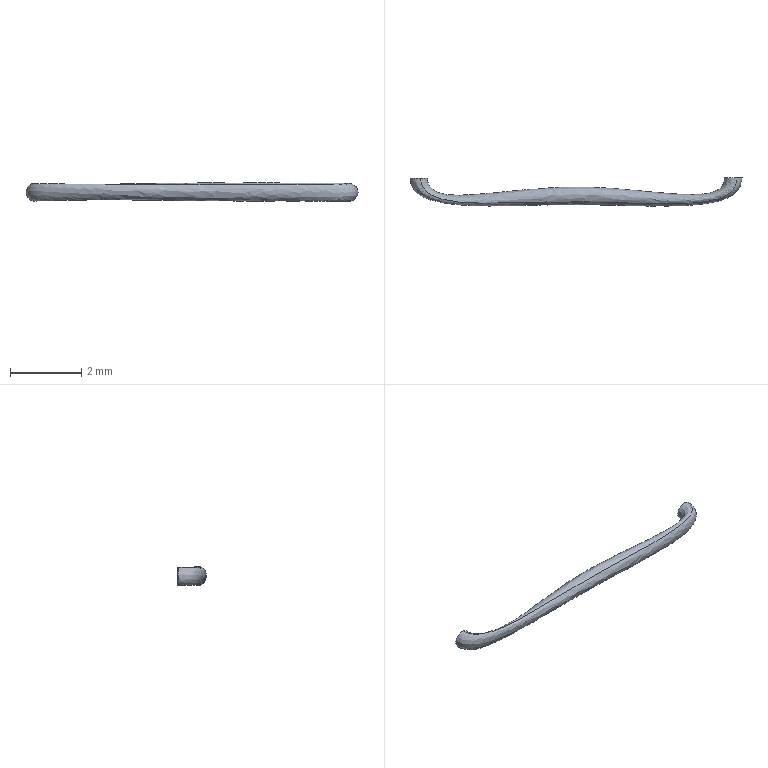Part | SolidWorks | features BaseBody 1 | 1 solid | 4 faces | box 9.341 x 0.7921 x 0.5174 mm | volume 1.419 mm3 | plane 2 | spline 2
STEP:
#1=CARTESIAN_POINT('',(346.48,392.468,97.127));
#2=VERTEX_POINT('',#1);
#3=CARTESIAN_POINT('',(346.268,392.468,96.674));
#4=VERTEX_POINT('',#3);
#5=CARTESIAN_POINT('',(346.48,392.468,97.127));
#6=CARTESIAN_POINT('',(346.486,392.468,97.124));
#7=CARTESIAN_POINT('',(346.498,392.468,97.117));
#8=CARTESIAN_POINT('',(346.515,392.468,97.107));
#9=CARTESIAN_POINT('',(346.531,392.468,97.095));
#10=CARTESIAN_POINT('',(346.581,392.468,97.051));
#11=CARTESIAN_POINT('',(346.622,392.469,96.975));
#12=CARTESIAN_POINT('',(346.626,392.469,96.871));
#13=CARTESIAN_POINT('',(346.602,392.469,96.785));
#14=CARTESIAN_POINT('',(346.545,392.468,96.709));
#15=CARTESIAN_POINT('',(346.461,392.468,96.66));
#16=CARTESIAN_POINT('',(346.365,392.468,96.644));
#17=CARTESIAN_POINT('',(346.298,392.468,96.66));
#18=CARTESIAN_POINT('',(346.268,392.468,96.674));
#19=B_SPLINE_CURVE_WITH_KNOTS('',3,(#5,#6,#7,#8,#9,#10,#11,#12,#13,#14,#15,#16,#17,#18),.UNSPECIFIED.,.F.,.F.,(4,1,1,1,1,1,1,1,1,1,1,4),(0.,0.025,0.05,0.075,0.1,0.3,0.4,0.5,0.625,0.75,0.875,1.),.UNSPECIFIED.);
#20=EDGE_CURVE('',#2,#4,#19,.T.);
#21=ORIENTED_EDGE('',*,*,#20,.T.);
#22=CARTESIAN_POINT('',(346.268,392.468,96.674));
#23=CARTESIAN_POINT('',(346.237,392.468,96.688));
#24=CARTESIAN_POINT('',(346.182,392.468,96.729));
#25=CARTESIAN_POINT('',(346.133,392.468,96.813));
#26=CARTESIAN_POINT('',(346.117,392.468,96.909));
#27=CARTESIAN_POINT('',(346.14,392.468,97.002));
#28=CARTESIAN_POINT('',(346.19,392.468,97.076));
#29=CARTESIAN_POINT('',(346.273,392.468,97.139));
#30=CARTESIAN_POINT('',(346.358,392.468,97.156));
#31=CARTESIAN_POINT('',(346.423,392.468,97.146));
#32=CARTESIAN_POINT('',(346.442,392.468,97.141));
#33=CARTESIAN_POINT('',(346.461,392.468,97.135));
#34=CARTESIAN_POINT('',(346.474,392.468,97.129));
#35=CARTESIAN_POINT('',(346.48,392.468,97.127));
#36=B_SPLINE_CURVE_WITH_KNOTS('',3,(#22,#23,#24,#25,#26,#27,#28,#29,#30,#31,#32,#33,#34,#35),.UNSPECIFIED.,.F.,.F.,(4,1,1,1,1,1,1,1,1,1,1,4),(0.,0.125,0.25,0.375,0.5,0.6,0.7,0.9,0.925,0.95,0.975,1.),.UNSPECIFIED.);
#37=EDGE_CURVE('',#4,#2,#36,.T.);
#38=ORIENTED_EDGE('',*,*,#37,.T.);
#39=EDGE_LOOP('',(#21,#38));
#40=FACE_OUTER_BOUND('',#39,.T.);
#41=CARTESIAN_POINT('',(346.374,392.468,96.9));
#42=DIRECTION('',(0.0009599,-1.,0.));
#43=DIRECTION('',(0.,0.,-1.));
#44=AXIS2_PLACEMENT_3D('',#41,#42,#43);
#45=PLANE('',#44);
#46=ADVANCED_FACE('',(#40),#45,.F.);
#47=CARTESIAN_POINT('',(337.585,392.46,97.145));
#48=VERTEX_POINT('',#47);
#49=CARTESIAN_POINT('',(337.481,392.46,96.656));
#50=VERTEX_POINT('',#49);
#51=CARTESIAN_POINT('',(337.585,392.46,97.145));
#52=CARTESIAN_POINT('',(337.591,392.46,97.143));
#53=CARTESIAN_POINT('',(337.605,392.46,97.14));
#54=CARTESIAN_POINT('',(337.624,392.46,97.133));
#55=CARTESIAN_POINT('',(337.642,392.46,97.125));
#56=CARTESIAN_POINT('',(337.7,392.46,97.094));
#57=CARTESIAN_POINT('',(337.757,392.46,97.029));
#58=CARTESIAN_POINT('',(337.785,392.46,96.929));
#59=CARTESIAN_POINT('',(337.781,392.46,96.84));
#60=CARTESIAN_POINT('',(337.743,392.46,96.753));
#61=CARTESIAN_POINT('',(337.672,392.46,96.686));
#62=CARTESIAN_POINT('',(337.582,392.46,96.648));
#63=CARTESIAN_POINT('',(337.514,392.46,96.649));
#64=CARTESIAN_POINT('',(337.481,392.46,96.656));
#65=B_SPLINE_CURVE_WITH_KNOTS('',3,(#51,#52,#53,#54,#55,#56,#57,#58,#59,#60,#61,#62,#63,#64),.UNSPECIFIED.,.F.,.F.,(4,1,1,1,1,1,1,1,1,1,1,4),(0.,0.025,0.05,0.075,0.1,0.3,0.4,0.5,0.625,0.75,0.875,1.),.UNSPECIFIED.);
#66=EDGE_CURVE('',#48,#50,#65,.T.);
#67=ORIENTED_EDGE('',*,*,#66,.T.);
#68=CARTESIAN_POINT('',(337.481,392.46,96.656));
#69=CARTESIAN_POINT('',(337.448,392.46,96.663));
#70=CARTESIAN_POINT('',(337.385,392.46,96.69));
#71=CARTESIAN_POINT('',(337.318,392.46,96.761));
#72=CARTESIAN_POINT('',(337.281,392.46,96.851));
#73=CARTESIAN_POINT('',(337.281,392.46,96.947));
#74=CARTESIAN_POINT('',(337.314,392.46,97.029));
#75=CARTESIAN_POINT('',(337.38,392.46,97.109));
#76=CARTESIAN_POINT('',(337.459,392.46,97.146));
#77=CARTESIAN_POINT('',(337.524,392.46,97.15));
#78=CARTESIAN_POINT('',(337.544,392.46,97.15));
#79=CARTESIAN_POINT('',(337.564,392.46,97.148));
#80=CARTESIAN_POINT('',(337.578,392.46,97.146));
#81=CARTESIAN_POINT('',(337.585,392.46,97.145));
#82=B_SPLINE_CURVE_WITH_KNOTS('',3,(#68,#69,#70,#71,#72,#73,#74,#75,#76,#77,#78,#79,#80,#81),.UNSPECIFIED.,.F.,.F.,(4,1,1,1,1,1,1,1,1,1,1,4),(0.,0.125,0.25,0.375,0.5,0.6,0.7,0.9,0.925,0.95,0.975,1.),.UNSPECIFIED.);
#83=EDGE_CURVE('',#50,#48,#82,.T.);
#84=ORIENTED_EDGE('',*,*,#83,.T.);
#85=EDGE_LOOP('',(#67,#84));
#86=FACE_OUTER_BOUND('',#85,.T.);
#87=CARTESIAN_POINT('',(337.533,392.46,96.9));
#88=DIRECTION('',(0.0009599,-1.,0.));
#89=DIRECTION('',(0.,0.,-1.));
#90=AXIS2_PLACEMENT_3D('',#87,#88,#89);
#91=PLANE('',#90);
#92=ADVANCED_FACE('',(#86),#91,.F.);
#93=CARTESIAN_POINT('',(337.481,392.46,96.656));
#94=CARTESIAN_POINT('',(337.482,391.517,96.656));
#95=CARTESIAN_POINT('',(342.031,392.705,96.768));
#96=CARTESIAN_POINT('',(346.269,391.557,96.674));
#97=CARTESIAN_POINT('',(346.268,392.468,96.674));
#98=B_SPLINE_CURVE_WITH_KNOTS('',3,(#93,#94,#95,#96,#97),.UNSPECIFIED.,.F.,.F.,(4,1,4),(0.,0.5,1.),.UNSPECIFIED.);
#99=EDGE_CURVE('',#50,#4,#98,.T.);
#100=ORIENTED_EDGE('',*,*,#99,.T.);
#101=ORIENTED_EDGE('',*,*,#20,.F.);
#102=CARTESIAN_POINT('',(346.48,392.468,97.127));
#103=CARTESIAN_POINT('',(346.481,391.466,97.127));
#104=CARTESIAN_POINT('',(341.874,392.138,97.077));
#105=CARTESIAN_POINT('',(337.586,391.489,97.145));
#106=CARTESIAN_POINT('',(337.585,392.46,97.145));
#107=B_SPLINE_CURVE_WITH_KNOTS('',3,(#102,#103,#104,#105,#106),.UNSPECIFIED.,.F.,.F.,(4,1,4),(0.,0.5,1.),.UNSPECIFIED.);
#108=EDGE_CURVE('',#2,#48,#107,.T.);
#109=ORIENTED_EDGE('',*,*,#108,.T.);
#110=ORIENTED_EDGE('',*,*,#83,.F.);
#111=EDGE_LOOP('',(#100,#101,#109,#110));
#112=FACE_OUTER_BOUND('',#111,.T.);
#113=CARTESIAN_POINT('',(337.606,392.553,97.141));
#114=CARTESIAN_POINT('',(337.469,391.473,97.142));
#115=CARTESIAN_POINT('',(341.873,392.18,97.093));
#116=CARTESIAN_POINT('',(346.619,391.448,97.134));
#117=CARTESIAN_POINT('',(346.458,392.572,97.133));
#118=CARTESIAN_POINT('',(337.601,392.553,97.142));
#119=CARTESIAN_POINT('',(337.464,391.471,97.144));
#120=CARTESIAN_POINT('',(341.873,392.173,97.087));
#121=CARTESIAN_POINT('',(346.624,391.446,97.132));
#122=CARTESIAN_POINT('',(346.463,392.572,97.131));
#123=CARTESIAN_POINT('',(337.589,392.554,97.145));
#124=CARTESIAN_POINT('',(337.451,391.468,97.147));
#125=CARTESIAN_POINT('',(341.873,392.157,97.073));
#126=CARTESIAN_POINT('',(346.635,391.443,97.128));
#127=CARTESIAN_POINT('',(346.474,392.572,97.126));
#128=CARTESIAN_POINT('',(337.57,392.554,97.148));
#129=CARTESIAN_POINT('',(337.432,391.462,97.151));
#130=CARTESIAN_POINT('',(341.874,392.133,97.05));
#131=CARTESIAN_POINT('',(346.652,391.438,97.119));
#132=CARTESIAN_POINT('',(346.491,392.573,97.117));
#133=CARTESIAN_POINT('',(337.55,392.555,97.15));
#134=CARTESIAN_POINT('',(337.411,391.456,97.154));
#135=CARTESIAN_POINT('',(341.876,392.111,97.025));
#136=CARTESIAN_POINT('',(346.67,391.433,97.109));
#137=CARTESIAN_POINT('',(346.508,392.574,97.106));
#138=CARTESIAN_POINT('',(337.53,392.555,97.15));
#139=CARTESIAN_POINT('',(337.391,391.451,97.155));
#140=CARTESIAN_POINT('',(341.878,392.09,97.));
#141=CARTESIAN_POINT('',(346.686,391.428,97.098));
#142=CARTESIAN_POINT('',(346.524,392.574,97.094));
#143=CARTESIAN_POINT('',(337.465,392.557,97.145));
#144=CARTESIAN_POINT('',(337.323,391.433,97.153));
#145=CARTESIAN_POINT('',(341.887,392.031,96.914));
#146=CARTESIAN_POINT('',(346.737,391.414,97.056));
#147=CARTESIAN_POINT('',(346.573,392.576,97.051));
#148=CARTESIAN_POINT('',(337.386,392.559,97.109));
#149=CARTESIAN_POINT('',(337.241,391.413,97.119));
#150=CARTESIAN_POINT('',(341.907,392.003,96.801));
#151=CARTESIAN_POINT('',(346.779,391.403,96.981));
#152=CARTESIAN_POINT('',(346.614,392.577,96.975));
#153=CARTESIAN_POINT('',(337.32,392.56,97.029));
#154=CARTESIAN_POINT('',(337.172,391.402,97.04));
#155=CARTESIAN_POINT('',(341.94,392.048,96.688));
#156=CARTESIAN_POINT('',(346.783,391.404,96.877));
#157=CARTESIAN_POINT('',(346.619,392.577,96.871));
#158=CARTESIAN_POINT('',(337.288,392.56,96.946));
#159=CARTESIAN_POINT('',(337.138,391.4,96.957));
#160=CARTESIAN_POINT('',(341.97,392.132,96.618));
#161=CARTESIAN_POINT('',(346.757,391.413,96.791));
#162=CARTESIAN_POINT('',(346.595,392.576,96.785));
#163=CARTESIAN_POINT('',(337.288,392.559,96.85));
#164=CARTESIAN_POINT('',(337.136,391.409,96.859));
#165=CARTESIAN_POINT('',(342.001,392.266,96.584));
#166=CARTESIAN_POINT('',(346.696,391.432,96.713));
#167=CARTESIAN_POINT('',(346.537,392.573,96.709));
#168=CARTESIAN_POINT('',(337.325,392.557,96.761));
#169=CARTESIAN_POINT('',(337.174,391.428,96.766));
#170=CARTESIAN_POINT('',(342.025,392.428,96.6));
#171=CARTESIAN_POINT('',(346.609,391.461,96.661));
#172=CARTESIAN_POINT('',(346.453,392.57,96.659));
#173=CARTESIAN_POINT('',(337.392,392.554,96.69));
#174=CARTESIAN_POINT('',(337.242,391.453,96.691));
#175=CARTESIAN_POINT('',(342.041,392.595,96.661));
#176=CARTESIAN_POINT('',(346.509,391.491,96.643));
#177=CARTESIAN_POINT('',(346.357,392.567,96.644));
#178=CARTESIAN_POINT('',(337.459,392.552,96.661));
#179=CARTESIAN_POINT('',(337.312,391.472,96.658));
#180=CARTESIAN_POINT('',(342.043,392.707,96.737));
#181=CARTESIAN_POINT('',(346.435,391.511,96.658));
#182=CARTESIAN_POINT('',(346.286,392.564,96.661));
#183=CARTESIAN_POINT('',(337.497,392.551,96.654));
#184=CARTESIAN_POINT('',(337.351,391.482,96.65));
#185=CARTESIAN_POINT('',(342.041,392.756,96.784));
#186=CARTESIAN_POINT('',(346.399,391.521,96.675));
#187=CARTESIAN_POINT('',(346.251,392.563,96.678));
#188=CARTESIAN_POINT('',(337.502,392.551,96.653));
#189=CARTESIAN_POINT('',(337.357,391.483,96.649));
#190=CARTESIAN_POINT('',(342.04,392.762,96.79));
#191=CARTESIAN_POINT('',(346.394,391.522,96.677));
#192=CARTESIAN_POINT('',(346.247,392.563,96.681));
#193=B_SPLINE_SURFACE_WITH_KNOTS('',3,3,((#113,#114,#115,#116,#117),(#118,#119,#120,#121,#122),(#123,#124,#125,#126,#127),(#128,#129,#130,#131,#132),(#133,#134,#135,#136,#137),(#138,#139,#140,#141,#142),(#143,#144,#145,#146,#147),(#148,#149,#150,#151,#152),(#153,#154,#155,#156,#157),(#158,#159,#160,#161,#162),(#163,#164,#165,#166,#167),(#168,#169,#170,#171,#172),(#173,#174,#175,#176,#177),(#178,#179,#180,#181,#182),(#183,#184,#185,#186,#187),(#188,#189,#190,#191,#192)),.UNSPECIFIED.,.F.,.F.,.F.,(4,1,1,1,1,1,1,1,1,1,1,1,1,4),(4,1,4),(-0.009538,0.,0.0125,0.025,0.0375,0.05,0.15,0.2,0.25,0.3125,0.375,0.4375,0.5,0.5095),(-0.01545,0.5,1.017),.UNSPECIFIED.);
#194=ADVANCED_FACE('',(#112),#193,.T.);
#195=ORIENTED_EDGE('',*,*,#66,.F.);
#196=ORIENTED_EDGE('',*,*,#108,.F.);
#197=ORIENTED_EDGE('',*,*,#37,.F.);
#198=ORIENTED_EDGE('',*,*,#99,.F.);
#199=EDGE_LOOP('',(#195,#196,#197,#198));
#200=FACE_OUTER_BOUND('',#199,.T.);
#201=CARTESIAN_POINT('',(337.472,392.552,96.659));
#202=CARTESIAN_POINT('',(337.326,391.476,96.656));
#203=CARTESIAN_POINT('',(342.042,392.722,96.754));
#204=CARTESIAN_POINT('',(346.423,391.514,96.665));
#205=CARTESIAN_POINT('',(346.275,392.564,96.668));
#206=CARTESIAN_POINT('',(337.477,392.552,96.658));
#207=CARTESIAN_POINT('',(337.331,391.477,96.655));
#208=CARTESIAN_POINT('',(342.042,392.729,96.76));
#209=CARTESIAN_POINT('',(346.418,391.516,96.667));
#210=CARTESIAN_POINT('',(346.27,392.564,96.67));
#211=CARTESIAN_POINT('',(337.515,392.551,96.649));
#212=CARTESIAN_POINT('',(337.369,391.487,96.644));
#213=CARTESIAN_POINT('',(342.04,392.781,96.804));
#214=CARTESIAN_POINT('',(346.382,391.525,96.681));
#215=CARTESIAN_POINT('',(346.234,392.563,96.685));
#216=CARTESIAN_POINT('',(337.588,392.549,96.649));
#217=CARTESIAN_POINT('',(337.446,391.505,96.641));
#218=CARTESIAN_POINT('',(342.032,392.858,96.899));
#219=CARTESIAN_POINT('',(346.321,391.54,96.724));
#220=CARTESIAN_POINT('',(346.175,392.561,96.729));
#221=CARTESIAN_POINT('',(337.678,392.547,96.686));
#222=CARTESIAN_POINT('',(337.539,391.526,96.675));
#223=CARTESIAN_POINT('',(342.011,392.897,97.027));
#224=CARTESIAN_POINT('',(346.271,391.553,96.806));
#225=CARTESIAN_POINT('',(346.126,392.56,96.814));
#226=CARTESIAN_POINT('',(337.749,392.546,96.753));
#227=CARTESIAN_POINT('',(337.613,391.541,96.741));
#228=CARTESIAN_POINT('',(341.981,392.873,97.14));
#229=CARTESIAN_POINT('',(346.255,391.556,96.902));
#230=CARTESIAN_POINT('',(346.11,392.559,96.91));
#231=CARTESIAN_POINT('',(337.787,392.546,96.841));
#232=CARTESIAN_POINT('',(337.653,391.546,96.829));
#233=CARTESIAN_POINT('',(341.949,392.787,97.22));
#234=CARTESIAN_POINT('',(346.279,391.55,96.995));
#235=CARTESIAN_POINT('',(346.132,392.56,97.003));
#236=CARTESIAN_POINT('',(337.791,392.546,96.93));
#237=CARTESIAN_POINT('',(337.658,391.541,96.919));
#238=CARTESIAN_POINT('',(341.92,392.664,97.256));
#239=CARTESIAN_POINT('',(346.332,391.535,97.07));
#240=CARTESIAN_POINT('',(346.183,392.562,97.076));
#241=CARTESIAN_POINT('',(337.763,392.548,97.03));
#242=CARTESIAN_POINT('',(337.63,391.526,97.022));
#243=CARTESIAN_POINT('',(341.891,392.495,97.255));
#244=CARTESIAN_POINT('',(346.419,391.508,97.135));
#245=CARTESIAN_POINT('',(346.265,392.565,97.139));
#246=CARTESIAN_POINT('',(337.706,392.55,97.094));
#247=CARTESIAN_POINT('',(337.572,391.505,97.091));
#248=CARTESIAN_POINT('',(341.877,392.346,97.205));
#249=CARTESIAN_POINT('',(346.507,391.481,97.154));
#250=CARTESIAN_POINT('',(346.35,392.568,97.156));
#251=CARTESIAN_POINT('',(337.648,392.552,97.125));
#252=CARTESIAN_POINT('',(337.512,391.486,97.125));
#253=CARTESIAN_POINT('',(341.873,392.244,97.141));
#254=CARTESIAN_POINT('',(346.574,391.461,97.146));
#255=CARTESIAN_POINT('',(346.415,392.57,97.146));
#256=CARTESIAN_POINT('',(337.63,392.552,97.133));
#257=CARTESIAN_POINT('',(337.493,391.48,97.134));
#258=CARTESIAN_POINT('',(341.873,392.214,97.121));
#259=CARTESIAN_POINT('',(346.594,391.455,97.142));
#260=CARTESIAN_POINT('',(346.434,392.571,97.141));
#261=CARTESIAN_POINT('',(337.611,392.553,97.14));
#262=CARTESIAN_POINT('',(337.474,391.474,97.141));
#263=CARTESIAN_POINT('',(341.873,392.186,97.099));
#264=CARTESIAN_POINT('',(346.614,391.449,97.136));
#265=CARTESIAN_POINT('',(346.453,392.572,97.135));
#266=CARTESIAN_POINT('',(337.592,392.554,97.144));
#267=CARTESIAN_POINT('',(337.455,391.469,97.147));
#268=CARTESIAN_POINT('',(341.873,392.161,97.077));
#269=CARTESIAN_POINT('',(346.632,391.444,97.129));
#270=CARTESIAN_POINT('',(346.471,392.572,97.127));
#271=CARTESIAN_POINT('',(337.58,392.554,97.147));
#272=CARTESIAN_POINT('',(337.442,391.465,97.149));
#273=CARTESIAN_POINT('',(341.874,392.146,97.062));
#274=CARTESIAN_POINT('',(346.643,391.441,97.124));
#275=CARTESIAN_POINT('',(346.482,392.573,97.122));
#276=CARTESIAN_POINT('',(337.575,392.554,97.147));
#277=CARTESIAN_POINT('',(337.437,391.464,97.15));
#278=CARTESIAN_POINT('',(341.874,392.14,97.056));
#279=CARTESIAN_POINT('',(346.648,391.439,97.121));
#280=CARTESIAN_POINT('',(346.486,392.573,97.119));
#281=B_SPLINE_SURFACE_WITH_KNOTS('',3,3,((#201,#202,#203,#204,#205),(#206,#207,#208,#209,#210),(#211,#212,#213,#214,#215),(#216,#217,#218,#219,#220),(#221,#222,#223,#224,#225),(#226,#227,#228,#229,#230),(#231,#232,#233,#234,#235),(#236,#237,#238,#239,#240),(#241,#242,#243,#244,#245),(#246,#247,#248,#249,#250),(#251,#252,#253,#254,#255),(#256,#257,#258,#259,#260),(#261,#262,#263,#264,#265),(#266,#267,#268,#269,#270),(#271,#272,#273,#274,#275),(#276,#277,#278,#279,#280)),.UNSPECIFIED.,.F.,.F.,.F.,(4,1,1,1,1,1,1,1,1,1,1,1,1,4),(4,1,4),(0.4905,0.5,0.5625,0.625,0.6875,0.75,0.8,0.85,0.95,0.9625,0.975,0.9875,1.,1.01),(-0.01545,0.5,1.017),.UNSPECIFIED.);
#282=ADVANCED_FACE('',(#200),#281,.T.);
#283=CLOSED_SHELL('',(#46,#92,#194,#282));
#284=MANIFOLD_SOLID_BREP('',#283);
#285=CARTESIAN_POINT('',(0.,0.,0.));
#286=DIRECTION('',(0.,0.,1.));
#287=DIRECTION('',(1.,0.,0.));
#288=AXIS2_PLACEMENT_3D('',#285,#286,#287);
#289=(LENGTH_UNIT()NAMED_UNIT(*)SI_UNIT(.MILLI.,.METRE.));
#290=UNCERTAINTY_MEASURE_WITH_UNIT(LENGTH_MEASURE(0.00001),#289,'','');
#291=(NAMED_UNIT(*)PLANE_ANGLE_UNIT()SI_UNIT($,.RADIAN.));
#292=(NAMED_UNIT(*)SI_UNIT($,.STERADIAN.)SOLID_ANGLE_UNIT());
#293=(GEOMETRIC_REPRESENTATION_CONTEXT(3)GLOBAL_UNCERTAINTY_ASSIGNED_CONTEXT((#290))GLOBAL_UNIT_ASSIGNED_CONTEXT((#289,#291,#292))REPRESENTATION_CONTEXT('',''));
#294=ADVANCED_BREP_SHAPE_REPRESENTATION('',(#284,#288),#293);